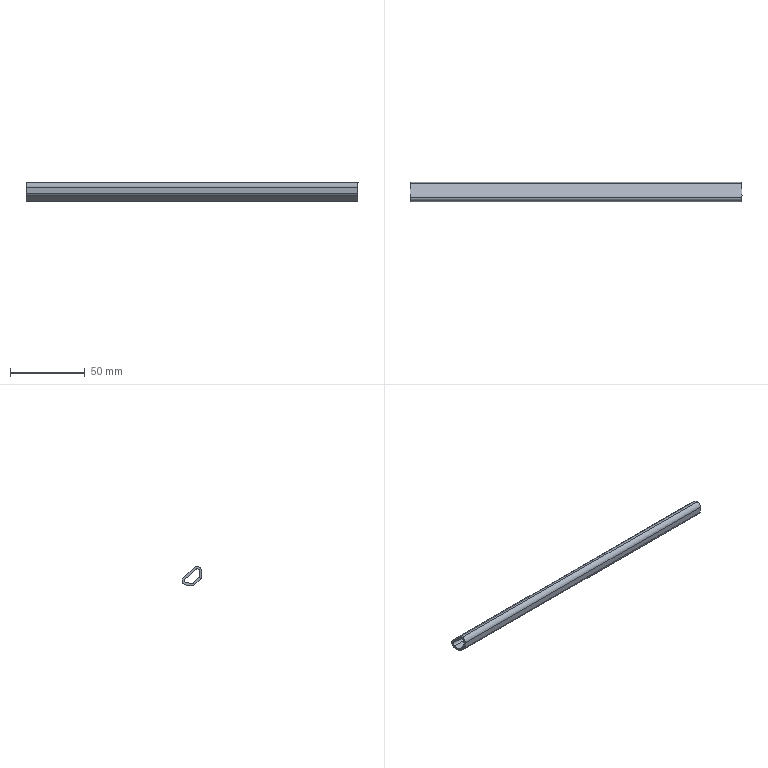Part | SolidWorks | features BaseBody 1 | 1 solid | 20 faces | box 221.8 x 13.077 x 12.577 mm | volume 11773 mm3 | plane 10 | cylinder 10 | commonest cylinder face diameters 3 x3 6 x3 1 x2 4 x2
STEP:
#1=CARTESIAN_POINT('',(110.837,-148.389,-339.63));
#2=VERTEX_POINT('',#1);
#3=CARTESIAN_POINT('',(-110.963,-148.389,-339.63));
#4=VERTEX_POINT('',#3);
#5=CARTESIAN_POINT('',(110.837,-148.389,-339.63));
#6=DIRECTION('',(-1.,0.000000003,0.000000006));
#7=VECTOR('',#6,1000.);
#8=LINE('',#5,#7);
#9=EDGE_CURVE('',#2,#4,#8,.T.);
#10=ORIENTED_EDGE('',*,*,#9,.F.);
#11=CARTESIAN_POINT('',(110.837,-144.347,-339.415));
#12=VERTEX_POINT('',#11);
#13=CARTESIAN_POINT('',(110.837,-144.347,-339.415));
#14=DIRECTION('',(-0.000000003,-0.9986,-0.05296));
#15=VECTOR('',#14,1000.);
#16=LINE('',#13,#15);
#17=EDGE_CURVE('',#12,#2,#16,.T.);
#18=ORIENTED_EDGE('',*,*,#17,.F.);
#19=CARTESIAN_POINT('',(-110.963,-144.347,-339.415));
#20=VERTEX_POINT('',#19);
#21=CARTESIAN_POINT('',(110.837,-144.347,-339.415));
#22=DIRECTION('',(-1.,0.000000003,0.000000006));
#23=VECTOR('',#22,1000.);
#24=LINE('',#21,#23);
#25=EDGE_CURVE('',#12,#20,#24,.T.);
#26=ORIENTED_EDGE('',*,*,#25,.T.);
#27=CARTESIAN_POINT('',(-110.963,-144.347,-339.415));
#28=DIRECTION('',(-0.000000003,-0.9986,-0.05296));
#29=VECTOR('',#28,1000.);
#30=LINE('',#27,#29);
#31=EDGE_CURVE('',#20,#4,#30,.T.);
#32=ORIENTED_EDGE('',*,*,#31,.T.);
#33=EDGE_LOOP('',(#10,#18,#26,#32));
#34=FACE_OUTER_BOUND('',#33,.T.);
#35=CARTESIAN_POINT('',(-110.563,-144.347,-339.415));
#36=DIRECTION('',(0.000000006,-0.05296,0.9986));
#37=DIRECTION('',(-1.,-0.000000113,0.));
#38=AXIS2_PLACEMENT_3D('',#35,#36,#37);
#39=PLANE('',#38);
#40=ADVANCED_FACE('',(#34),#39,.T.);
#41=CARTESIAN_POINT('',(-110.963,-150.5,-330.438));
#42=VERTEX_POINT('',#41);
#43=CARTESIAN_POINT('',(-110.963,-143.423,-336.802));
#44=VERTEX_POINT('',#43);
#45=CARTESIAN_POINT('',(-110.963,-150.5,-330.438));
#46=DIRECTION('',(-0.000000002,0.7436,-0.6687));
#47=VECTOR('',#46,1000.);
#48=LINE('',#45,#47);
#49=EDGE_CURVE('',#42,#44,#48,.T.);
#50=ORIENTED_EDGE('',*,*,#49,.F.);
#51=CARTESIAN_POINT('',(-110.963,-151.583,-330.055));
#52=VERTEX_POINT('',#51);
#53=CARTESIAN_POINT('',(-110.963,-151.503,-331.553));
#54=DIRECTION('',(-1.,0.000000003,0.000000006));
#55=DIRECTION('',(0.000000006,-0.05296,0.9986));
#56=AXIS2_PLACEMENT_3D('',#53,#54,#55);
#57=CIRCLE('',#56,1.5);
#58=EDGE_CURVE('',#52,#42,#57,.T.);
#59=ORIENTED_EDGE('',*,*,#58,.F.);
#60=CARTESIAN_POINT('',(-110.963,-153.001,-331.633));
#61=VERTEX_POINT('',#60);
#62=CARTESIAN_POINT('',(-110.963,-151.503,-331.553));
#63=DIRECTION('',(-1.,0.000000003,0.000000006));
#64=DIRECTION('',(0.000000006,-0.05296,0.9986));
#65=AXIS2_PLACEMENT_3D('',#62,#63,#64);
#66=CIRCLE('',#65,1.5);
#67=EDGE_CURVE('',#61,#52,#66,.T.);
#68=ORIENTED_EDGE('',*,*,#67,.F.);
#69=CARTESIAN_POINT('',(-110.963,-152.787,-335.675));
#70=VERTEX_POINT('',#69);
#71=CARTESIAN_POINT('',(-110.963,-152.787,-335.675));
#72=DIRECTION('',(0.000000006,-0.05296,0.9986));
#73=VECTOR('',#72,1000.);
#74=LINE('',#71,#73);
#75=EDGE_CURVE('',#70,#61,#74,.T.);
#76=ORIENTED_EDGE('',*,*,#75,.F.);
#77=CARTESIAN_POINT('',(-110.963,-152.622,-336.021));
#78=VERTEX_POINT('',#77);
#79=CARTESIAN_POINT('',(-110.963,-152.287,-335.649));
#80=DIRECTION('',(-1.,0.000000003,0.000000006));
#81=DIRECTION('',(-0.000000006,-0.6687,-0.7436));
#82=AXIS2_PLACEMENT_3D('',#79,#80,#81);
#83=CIRCLE('',#82,0.5);
#84=EDGE_CURVE('',#78,#70,#83,.T.);
#85=ORIENTED_EDGE('',*,*,#84,.F.);
#86=CARTESIAN_POINT('',(-110.963,-148.75,-339.502));
#87=VERTEX_POINT('',#86);
#88=CARTESIAN_POINT('',(-110.963,-148.75,-339.502));
#89=DIRECTION('',(0.000000002,-0.7436,0.6687));
#90=VECTOR('',#89,1000.);
#91=LINE('',#88,#90);
#92=EDGE_CURVE('',#87,#78,#91,.T.);
#93=ORIENTED_EDGE('',*,*,#92,.F.);
#94=CARTESIAN_POINT('',(-110.963,-148.416,-339.13));
#95=DIRECTION('',(-1.,0.000000003,0.000000006));
#96=DIRECTION('',(-0.000000006,0.05296,-0.9986));
#97=AXIS2_PLACEMENT_3D('',#94,#95,#96);
#98=CIRCLE('',#97,0.5);
#99=EDGE_CURVE('',#4,#87,#98,.T.);
#100=ORIENTED_EDGE('',*,*,#99,.F.);
#101=ORIENTED_EDGE('',*,*,#31,.F.);
#102=CARTESIAN_POINT('',(-110.963,-144.426,-337.917));
#103=DIRECTION('',(-1.,0.000000003,0.000000006));
#104=DIRECTION('',(0.000000006,0.6687,0.7436));
#105=AXIS2_PLACEMENT_3D('',#102,#103,#104);
#106=CIRCLE('',#105,1.5);
#107=EDGE_CURVE('',#44,#20,#106,.T.);
#108=ORIENTED_EDGE('',*,*,#107,.F.);
#109=EDGE_LOOP('',(#50,#59,#68,#76,#85,#93,#100,#101,#108));
#110=FACE_BOUND('',#109,.T.);
#111=CARTESIAN_POINT('',(-110.963,-153.625,-337.136));
#112=VERTEX_POINT('',#111);
#113=CARTESIAN_POINT('',(-110.963,-149.753,-340.618));
#114=VERTEX_POINT('',#113);
#115=CARTESIAN_POINT('',(-110.963,-153.625,-337.136));
#116=DIRECTION('',(-0.000000002,0.7436,-0.6687));
#117=VECTOR('',#116,1000.);
#118=LINE('',#115,#117);
#119=EDGE_CURVE('',#112,#114,#118,.T.);
#120=ORIENTED_EDGE('',*,*,#119,.F.);
#121=CARTESIAN_POINT('',(-110.963,-154.285,-335.755));
#122=VERTEX_POINT('',#121);
#123=CARTESIAN_POINT('',(-110.963,-152.287,-335.649));
#124=DIRECTION('',(1.,-0.000000003,-0.000000006));
#125=DIRECTION('',(-0.000000003,-0.9986,-0.05296));
#126=AXIS2_PLACEMENT_3D('',#123,#124,#125);
#127=CIRCLE('',#126,2.);
#128=EDGE_CURVE('',#122,#112,#127,.T.);
#129=ORIENTED_EDGE('',*,*,#128,.F.);
#130=CARTESIAN_POINT('',(-110.963,-154.499,-331.712));
#131=VERTEX_POINT('',#130);
#132=CARTESIAN_POINT('',(-110.963,-154.499,-331.712));
#133=DIRECTION('',(-0.000000006,0.05296,-0.9986));
#134=VECTOR('',#133,1000.);
#135=LINE('',#132,#134);
#136=EDGE_CURVE('',#131,#122,#135,.T.);
#137=ORIENTED_EDGE('',*,*,#136,.F.);
#138=CARTESIAN_POINT('',(-110.963,-151.662,-328.557));
#139=VERTEX_POINT('',#138);
#140=CARTESIAN_POINT('',(-110.963,-151.503,-331.553));
#141=DIRECTION('',(1.,-0.000000003,-0.000000006));
#142=DIRECTION('',(0.000000006,-0.05296,0.9986));
#143=AXIS2_PLACEMENT_3D('',#140,#141,#142);
#144=CIRCLE('',#143,3.);
#145=EDGE_CURVE('',#139,#131,#144,.T.);
#146=ORIENTED_EDGE('',*,*,#145,.F.);
#147=CARTESIAN_POINT('',(-110.963,-149.497,-329.323));
#148=VERTEX_POINT('',#147);
#149=CARTESIAN_POINT('',(-110.963,-151.503,-331.553));
#150=DIRECTION('',(1.,-0.000000003,-0.000000006));
#151=DIRECTION('',(0.000000006,0.6687,0.7436));
#152=AXIS2_PLACEMENT_3D('',#149,#150,#151);
#153=CIRCLE('',#152,3.);
#154=EDGE_CURVE('',#148,#139,#153,.T.);
#155=ORIENTED_EDGE('',*,*,#154,.F.);
#156=CARTESIAN_POINT('',(-110.963,-142.42,-335.687));
#157=VERTEX_POINT('',#156);
#158=CARTESIAN_POINT('',(-110.963,-142.42,-335.687));
#159=DIRECTION('',(0.000000002,-0.7436,0.6687));
#160=VECTOR('',#159,1000.);
#161=LINE('',#158,#160);
#162=EDGE_CURVE('',#157,#148,#161,.T.);
#163=ORIENTED_EDGE('',*,*,#162,.F.);
#164=CARTESIAN_POINT('',(-110.963,-144.267,-340.913));
#165=VERTEX_POINT('',#164);
#166=CARTESIAN_POINT('',(-110.963,-144.426,-337.917));
#167=DIRECTION('',(1.,-0.000000003,-0.000000006));
#168=DIRECTION('',(-0.000000006,0.05296,-0.9986));
#169=AXIS2_PLACEMENT_3D('',#166,#167,#168);
#170=CIRCLE('',#169,3.);
#171=EDGE_CURVE('',#165,#157,#170,.T.);
#172=ORIENTED_EDGE('',*,*,#171,.F.);
#173=CARTESIAN_POINT('',(-110.963,-148.31,-341.128));
#174=VERTEX_POINT('',#173);
#175=CARTESIAN_POINT('',(-110.963,-148.31,-341.128));
#176=DIRECTION('',(0.000000003,0.9986,0.05296));
#177=VECTOR('',#176,1000.);
#178=LINE('',#175,#177);
#179=EDGE_CURVE('',#174,#165,#178,.T.);
#180=ORIENTED_EDGE('',*,*,#179,.F.);
#181=CARTESIAN_POINT('',(-110.963,-148.416,-339.13));
#182=DIRECTION('',(1.,-0.000000003,-0.000000006));
#183=DIRECTION('',(-0.000000006,-0.6687,-0.7436));
#184=AXIS2_PLACEMENT_3D('',#181,#182,#183);
#185=CIRCLE('',#184,2.);
#186=EDGE_CURVE('',#114,#174,#185,.T.);
#187=ORIENTED_EDGE('',*,*,#186,.F.);
#188=EDGE_LOOP('',(#120,#129,#137,#146,#155,#163,#172,#180,#187));
#189=FACE_OUTER_BOUND('',#188,.T.);
#190=CARTESIAN_POINT('',(-110.963,-148.416,-339.13));
#191=DIRECTION('',(1.,-0.000000003,-0.000000006));
#192=DIRECTION('',(0.,-0.9065,0.4222));
#193=AXIS2_PLACEMENT_3D('',#190,#191,#192);
#194=PLANE('',#193);
#195=ADVANCED_FACE('',(#110,#189),#194,.F.);
#196=CARTESIAN_POINT('',(110.837,-149.753,-340.618));
#197=VERTEX_POINT('',#196);
#198=CARTESIAN_POINT('',(110.837,-149.753,-340.618));
#199=DIRECTION('',(-1.,0.000000003,0.000000006));
#200=VECTOR('',#199,1000.);
#201=LINE('',#198,#200);
#202=EDGE_CURVE('',#197,#114,#201,.T.);
#203=ORIENTED_EDGE('',*,*,#202,.T.);
#204=ORIENTED_EDGE('',*,*,#186,.T.);
#205=CARTESIAN_POINT('',(110.837,-148.31,-341.128));
#206=VERTEX_POINT('',#205);
#207=CARTESIAN_POINT('',(110.837,-148.31,-341.128));
#208=DIRECTION('',(-1.,0.000000003,0.000000006));
#209=VECTOR('',#208,1000.);
#210=LINE('',#207,#209);
#211=EDGE_CURVE('',#206,#174,#210,.T.);
#212=ORIENTED_EDGE('',*,*,#211,.F.);
#213=CARTESIAN_POINT('',(110.837,-148.416,-339.13));
#214=DIRECTION('',(-1.,0.000000003,0.000000006));
#215=DIRECTION('',(-0.000000006,0.05296,-0.9986));
#216=AXIS2_PLACEMENT_3D('',#213,#214,#215);
#217=CIRCLE('',#216,2.);
#218=EDGE_CURVE('',#206,#197,#217,.T.);
#219=ORIENTED_EDGE('',*,*,#218,.T.);
#220=EDGE_LOOP('',(#203,#204,#212,#219));
#221=FACE_OUTER_BOUND('',#220,.T.);
#222=CARTESIAN_POINT('',(-110.563,-148.416,-339.13));
#223=DIRECTION('',(1.,-0.000000003,-0.000000006));
#224=DIRECTION('',(0.000000006,-0.05296,0.9986));
#225=AXIS2_PLACEMENT_3D('',#222,#223,#224);
#226=CYLINDRICAL_SURFACE('',#225,2.);
#227=ADVANCED_FACE('',(#221),#226,.T.);
#228=ORIENTED_EDGE('',*,*,#17,.T.);
#229=CARTESIAN_POINT('',(110.837,-148.75,-339.502));
#230=VERTEX_POINT('',#229);
#231=CARTESIAN_POINT('',(110.837,-148.416,-339.13));
#232=DIRECTION('',(1.,-0.000000003,-0.000000006));
#233=DIRECTION('',(-0.000000006,-0.6687,-0.7436));
#234=AXIS2_PLACEMENT_3D('',#231,#232,#233);
#235=CIRCLE('',#234,0.5);
#236=EDGE_CURVE('',#230,#2,#235,.T.);
#237=ORIENTED_EDGE('',*,*,#236,.F.);
#238=CARTESIAN_POINT('',(110.837,-152.622,-336.021));
#239=VERTEX_POINT('',#238);
#240=CARTESIAN_POINT('',(110.837,-152.622,-336.021));
#241=DIRECTION('',(-0.000000002,0.7436,-0.6687));
#242=VECTOR('',#241,1000.);
#243=LINE('',#240,#242);
#244=EDGE_CURVE('',#239,#230,#243,.T.);
#245=ORIENTED_EDGE('',*,*,#244,.F.);
#246=CARTESIAN_POINT('',(110.837,-152.787,-335.675));
#247=VERTEX_POINT('',#246);
#248=CARTESIAN_POINT('',(110.837,-152.287,-335.649));
#249=DIRECTION('',(1.,-0.000000003,-0.000000006));
#250=DIRECTION('',(-0.000000003,-0.9986,-0.05296));
#251=AXIS2_PLACEMENT_3D('',#248,#249,#250);
#252=CIRCLE('',#251,0.5);
#253=EDGE_CURVE('',#247,#239,#252,.T.);
#254=ORIENTED_EDGE('',*,*,#253,.F.);
#255=CARTESIAN_POINT('',(110.837,-153.001,-331.633));
#256=VERTEX_POINT('',#255);
#257=CARTESIAN_POINT('',(110.837,-152.787,-335.675));
#258=DIRECTION('',(0.000000006,-0.05296,0.9986));
#259=VECTOR('',#258,1000.);
#260=LINE('',#257,#259);
#261=EDGE_CURVE('',#247,#256,#260,.T.);
#262=ORIENTED_EDGE('',*,*,#261,.T.);
#263=CARTESIAN_POINT('',(110.837,-151.583,-330.055));
#264=VERTEX_POINT('',#263);
#265=CARTESIAN_POINT('',(110.837,-151.503,-331.553));
#266=DIRECTION('',(1.,-0.000000003,-0.000000006));
#267=DIRECTION('',(0.000000006,-0.05296,0.9986));
#268=AXIS2_PLACEMENT_3D('',#265,#266,#267);
#269=CIRCLE('',#268,1.5);
#270=EDGE_CURVE('',#264,#256,#269,.T.);
#271=ORIENTED_EDGE('',*,*,#270,.F.);
#272=CARTESIAN_POINT('',(110.837,-150.5,-330.438));
#273=VERTEX_POINT('',#272);
#274=CARTESIAN_POINT('',(110.837,-151.503,-331.553));
#275=DIRECTION('',(1.,-0.000000003,-0.000000006));
#276=DIRECTION('',(0.000000006,-0.05296,0.9986));
#277=AXIS2_PLACEMENT_3D('',#274,#275,#276);
#278=CIRCLE('',#277,1.5);
#279=EDGE_CURVE('',#273,#264,#278,.T.);
#280=ORIENTED_EDGE('',*,*,#279,.F.);
#281=CARTESIAN_POINT('',(110.837,-143.423,-336.802));
#282=VERTEX_POINT('',#281);
#283=CARTESIAN_POINT('',(110.837,-143.423,-336.802));
#284=DIRECTION('',(0.000000002,-0.7436,0.6687));
#285=VECTOR('',#284,1000.);
#286=LINE('',#283,#285);
#287=EDGE_CURVE('',#282,#273,#286,.T.);
#288=ORIENTED_EDGE('',*,*,#287,.F.);
#289=CARTESIAN_POINT('',(110.837,-144.426,-337.917));
#290=DIRECTION('',(1.,-0.000000003,-0.000000006));
#291=DIRECTION('',(-0.000000006,0.05296,-0.9986));
#292=AXIS2_PLACEMENT_3D('',#289,#290,#291);
#293=CIRCLE('',#292,1.5);
#294=EDGE_CURVE('',#12,#282,#293,.T.);
#295=ORIENTED_EDGE('',*,*,#294,.F.);
#296=EDGE_LOOP('',(#228,#237,#245,#254,#262,#271,#280,#288,#295));
#297=FACE_BOUND('',#296,.T.);
#298=CARTESIAN_POINT('',(110.837,-144.267,-340.913));
#299=VERTEX_POINT('',#298);
#300=CARTESIAN_POINT('',(110.837,-148.31,-341.128));
#301=DIRECTION('',(0.000000003,0.9986,0.05296));
#302=VECTOR('',#301,1000.);
#303=LINE('',#300,#302);
#304=EDGE_CURVE('',#206,#299,#303,.T.);
#305=ORIENTED_EDGE('',*,*,#304,.T.);
#306=CARTESIAN_POINT('',(110.837,-142.42,-335.687));
#307=VERTEX_POINT('',#306);
#308=CARTESIAN_POINT('',(110.837,-144.426,-337.917));
#309=DIRECTION('',(-1.,0.000000003,0.000000006));
#310=DIRECTION('',(0.000000006,0.6687,0.7436));
#311=AXIS2_PLACEMENT_3D('',#308,#309,#310);
#312=CIRCLE('',#311,3.);
#313=EDGE_CURVE('',#307,#299,#312,.T.);
#314=ORIENTED_EDGE('',*,*,#313,.F.);
#315=CARTESIAN_POINT('',(110.837,-149.497,-329.323));
#316=VERTEX_POINT('',#315);
#317=CARTESIAN_POINT('',(110.837,-149.497,-329.323));
#318=DIRECTION('',(-0.000000002,0.7436,-0.6687));
#319=VECTOR('',#318,1000.);
#320=LINE('',#317,#319);
#321=EDGE_CURVE('',#316,#307,#320,.T.);
#322=ORIENTED_EDGE('',*,*,#321,.F.);
#323=CARTESIAN_POINT('',(110.837,-151.662,-328.557));
#324=VERTEX_POINT('',#323);
#325=CARTESIAN_POINT('',(110.837,-151.503,-331.553));
#326=DIRECTION('',(-1.,0.000000003,0.000000006));
#327=DIRECTION('',(0.000000006,-0.05296,0.9986));
#328=AXIS2_PLACEMENT_3D('',#325,#326,#327);
#329=CIRCLE('',#328,3.);
#330=EDGE_CURVE('',#324,#316,#329,.T.);
#331=ORIENTED_EDGE('',*,*,#330,.F.);
#332=CARTESIAN_POINT('',(110.837,-154.499,-331.712));
#333=VERTEX_POINT('',#332);
#334=CARTESIAN_POINT('',(110.837,-151.503,-331.553));
#335=DIRECTION('',(-1.,0.000000003,0.000000006));
#336=DIRECTION('',(-0.000000003,-0.9986,-0.05296));
#337=AXIS2_PLACEMENT_3D('',#334,#335,#336);
#338=CIRCLE('',#337,3.);
#339=EDGE_CURVE('',#333,#324,#338,.T.);
#340=ORIENTED_EDGE('',*,*,#339,.F.);
#341=CARTESIAN_POINT('',(110.837,-154.285,-335.755));
#342=VERTEX_POINT('',#341);
#343=CARTESIAN_POINT('',(110.837,-154.499,-331.712));
#344=DIRECTION('',(-0.000000006,0.05296,-0.9986));
#345=VECTOR('',#344,1000.);
#346=LINE('',#343,#345);
#347=EDGE_CURVE('',#333,#342,#346,.T.);
#348=ORIENTED_EDGE('',*,*,#347,.T.);
#349=CARTESIAN_POINT('',(110.837,-153.625,-337.136));
#350=VERTEX_POINT('',#349);
#351=CARTESIAN_POINT('',(110.837,-152.287,-335.649));
#352=DIRECTION('',(-1.,0.000000003,0.000000006));
#353=DIRECTION('',(-0.000000006,-0.6687,-0.7436));
#354=AXIS2_PLACEMENT_3D('',#351,#352,#353);
#355=CIRCLE('',#354,2.);
#356=EDGE_CURVE('',#350,#342,#355,.T.);
#357=ORIENTED_EDGE('',*,*,#356,.F.);
#358=CARTESIAN_POINT('',(110.837,-149.753,-340.618));
#359=DIRECTION('',(0.000000002,-0.7436,0.6687));
#360=VECTOR('',#359,1000.);
#361=LINE('',#358,#360);
#362=EDGE_CURVE('',#197,#350,#361,.T.);
#363=ORIENTED_EDGE('',*,*,#362,.F.);
#364=ORIENTED_EDGE('',*,*,#218,.F.);
#365=EDGE_LOOP('',(#305,#314,#322,#331,#340,#348,#357,#363,#364));
#366=FACE_OUTER_BOUND('',#365,.T.);
#367=CARTESIAN_POINT('',(110.837,-148.416,-339.13));
#368=DIRECTION('',(1.,-0.000000003,-0.000000006));
#369=DIRECTION('',(0.,-0.9065,0.4222));
#370=AXIS2_PLACEMENT_3D('',#367,#368,#369);
#371=PLANE('',#370);
#372=ADVANCED_FACE('',(#297,#366),#371,.T.);
#373=CARTESIAN_POINT('',(110.837,-153.625,-337.136));
#374=DIRECTION('',(-1.,0.000000003,0.000000006));
#375=VECTOR('',#374,1000.);
#376=LINE('',#373,#375);
#377=EDGE_CURVE('',#350,#112,#376,.T.);
#378=ORIENTED_EDGE('',*,*,#377,.T.);
#379=ORIENTED_EDGE('',*,*,#119,.T.);
#380=ORIENTED_EDGE('',*,*,#202,.F.);
#381=ORIENTED_EDGE('',*,*,#362,.T.);
#382=EDGE_LOOP('',(#378,#379,#380,#381));
#383=FACE_OUTER_BOUND('',#382,.T.);
#384=CARTESIAN_POINT('',(-110.563,-149.753,-340.618));
#385=DIRECTION('',(0.000000006,0.6687,0.7436));
#386=DIRECTION('',(1.,-0.00000001,0.));
#387=AXIS2_PLACEMENT_3D('',#384,#385,#386);
#388=PLANE('',#387);
#389=ADVANCED_FACE('',(#383),#388,.F.);
#390=CARTESIAN_POINT('',(110.837,-154.285,-335.755));
#391=DIRECTION('',(-1.,0.000000003,0.000000006));
#392=VECTOR('',#391,1000.);
#393=LINE('',#390,#392);
#394=EDGE_CURVE('',#342,#122,#393,.T.);
#395=ORIENTED_EDGE('',*,*,#394,.T.);
#396=ORIENTED_EDGE('',*,*,#128,.T.);
#397=ORIENTED_EDGE('',*,*,#377,.F.);
#398=ORIENTED_EDGE('',*,*,#356,.T.);
#399=EDGE_LOOP('',(#395,#396,#397,#398));
#400=FACE_OUTER_BOUND('',#399,.T.);
#401=CARTESIAN_POINT('',(-110.563,-152.287,-335.649));
#402=DIRECTION('',(1.,-0.000000003,-0.000000006));
#403=DIRECTION('',(0.000000006,-0.05296,0.9986));
#404=AXIS2_PLACEMENT_3D('',#401,#402,#403);
#405=CYLINDRICAL_SURFACE('',#404,2.);
#406=ADVANCED_FACE('',(#400),#405,.T.);
#407=CARTESIAN_POINT('',(110.837,-154.499,-331.712));
#408=DIRECTION('',(-1.,0.000000003,0.000000006));
#409=VECTOR('',#408,1000.);
#410=LINE('',#407,#409);
#411=EDGE_CURVE('',#333,#131,#410,.T.);
#412=ORIENTED_EDGE('',*,*,#411,.T.);
#413=ORIENTED_EDGE('',*,*,#136,.T.);
#414=ORIENTED_EDGE('',*,*,#394,.F.);
#415=ORIENTED_EDGE('',*,*,#347,.F.);
#416=EDGE_LOOP('',(#412,#413,#414,#415));
#417=FACE_OUTER_BOUND('',#416,.T.);
#418=CARTESIAN_POINT('',(-110.563,-154.285,-335.755));
#419=DIRECTION('',(0.000000003,0.9986,0.05296));
#420=DIRECTION('',(1.,0.,-0.00000006));
#421=AXIS2_PLACEMENT_3D('',#418,#419,#420);
#422=PLANE('',#421);
#423=ADVANCED_FACE('',(#417),#422,.F.);
#424=ORIENTED_EDGE('',*,*,#145,.T.);
#425=ORIENTED_EDGE('',*,*,#411,.F.);
#426=ORIENTED_EDGE('',*,*,#339,.T.);
#427=CARTESIAN_POINT('',(110.837,-151.662,-328.557));
#428=DIRECTION('',(-1.,0.000000003,0.000000006));
#429=VECTOR('',#428,1000.);
#430=LINE('',#427,#429);
#431=EDGE_CURVE('',#324,#139,#430,.T.);
#432=ORIENTED_EDGE('',*,*,#431,.T.);
#433=EDGE_LOOP('',(#424,#425,#426,#432));
#434=FACE_OUTER_BOUND('',#433,.T.);
#435=CARTESIAN_POINT('',(-110.563,-151.503,-331.553));
#436=DIRECTION('',(1.,-0.000000003,-0.000000006));
#437=DIRECTION('',(0.000000006,-0.05296,0.9986));
#438=AXIS2_PLACEMENT_3D('',#435,#436,#437);
#439=CYLINDRICAL_SURFACE('',#438,3.);
#440=ADVANCED_FACE('',(#434),#439,.T.);
#441=ORIENTED_EDGE('',*,*,#431,.F.);
#442=ORIENTED_EDGE('',*,*,#330,.T.);
#443=CARTESIAN_POINT('',(110.837,-149.497,-329.323));
#444=DIRECTION('',(-1.,0.000000003,0.000000006));
#445=VECTOR('',#444,1000.);
#446=LINE('',#443,#445);
#447=EDGE_CURVE('',#316,#148,#446,.T.);
#448=ORIENTED_EDGE('',*,*,#447,.T.);
#449=ORIENTED_EDGE('',*,*,#154,.T.);
#450=EDGE_LOOP('',(#441,#442,#448,#449));
#451=FACE_OUTER_BOUND('',#450,.T.);
#452=CARTESIAN_POINT('',(-110.563,-151.503,-331.553));
#453=DIRECTION('',(1.,-0.000000003,-0.000000006));
#454=DIRECTION('',(0.000000006,-0.05296,0.9986));
#455=AXIS2_PLACEMENT_3D('',#452,#453,#454);
#456=CYLINDRICAL_SURFACE('',#455,3.);
#457=ADVANCED_FACE('',(#451),#456,.T.);
#458=CARTESIAN_POINT('',(110.837,-142.42,-335.687));
#459=DIRECTION('',(-1.,0.000000003,0.000000006));
#460=VECTOR('',#459,1000.);
#461=LINE('',#458,#460);
#462=EDGE_CURVE('',#307,#157,#461,.T.);
#463=ORIENTED_EDGE('',*,*,#462,.T.);
#464=ORIENTED_EDGE('',*,*,#162,.T.);
#465=ORIENTED_EDGE('',*,*,#447,.F.);
#466=ORIENTED_EDGE('',*,*,#321,.T.);
#467=EDGE_LOOP('',(#463,#464,#465,#466));
#468=FACE_OUTER_BOUND('',#467,.T.);
#469=CARTESIAN_POINT('',(-110.563,-142.42,-335.687));
#470=DIRECTION('',(0.000000006,0.6687,0.7436));
#471=DIRECTION('',(1.,-0.00000001,0.));
#472=AXIS2_PLACEMENT_3D('',#469,#470,#471);
#473=PLANE('',#472);
#474=ADVANCED_FACE('',(#468),#473,.T.);
#475=CARTESIAN_POINT('',(110.837,-144.267,-340.913));
#476=DIRECTION('',(-1.,0.000000003,0.000000006));
#477=VECTOR('',#476,1000.);
#478=LINE('',#475,#477);
#479=EDGE_CURVE('',#299,#165,#478,.T.);
#480=ORIENTED_EDGE('',*,*,#479,.T.);
#481=ORIENTED_EDGE('',*,*,#171,.T.);
#482=ORIENTED_EDGE('',*,*,#462,.F.);
#483=ORIENTED_EDGE('',*,*,#313,.T.);
#484=EDGE_LOOP('',(#480,#481,#482,#483));
#485=FACE_OUTER_BOUND('',#484,.T.);
#486=CARTESIAN_POINT('',(-110.563,-144.426,-337.917));
#487=DIRECTION('',(1.,-0.000000003,-0.000000006));
#488=DIRECTION('',(0.000000006,-0.05296,0.9986));
#489=AXIS2_PLACEMENT_3D('',#486,#487,#488);
#490=CYLINDRICAL_SURFACE('',#489,3.);
#491=ADVANCED_FACE('',(#485),#490,.T.);
#492=ORIENTED_EDGE('',*,*,#211,.T.);
#493=ORIENTED_EDGE('',*,*,#179,.T.);
#494=ORIENTED_EDGE('',*,*,#479,.F.);
#495=ORIENTED_EDGE('',*,*,#304,.F.);
#496=EDGE_LOOP('',(#492,#493,#494,#495));
#497=FACE_OUTER_BOUND('',#496,.T.);
#498=CARTESIAN_POINT('',(-110.563,-144.267,-340.913));
#499=DIRECTION('',(0.000000006,-0.05296,0.9986));
#500=DIRECTION('',(-1.,-0.000000113,0.));
#501=AXIS2_PLACEMENT_3D('',#498,#499,#500);
#502=PLANE('',#501);
#503=ADVANCED_FACE('',(#497),#502,.F.);
#504=ORIENTED_EDGE('',*,*,#25,.F.);
#505=ORIENTED_EDGE('',*,*,#294,.T.);
#506=CARTESIAN_POINT('',(110.837,-143.423,-336.802));
#507=DIRECTION('',(-1.,0.000000003,0.000000006));
#508=VECTOR('',#507,1000.);
#509=LINE('',#506,#508);
#510=EDGE_CURVE('',#282,#44,#509,.T.);
#511=ORIENTED_EDGE('',*,*,#510,.T.);
#512=ORIENTED_EDGE('',*,*,#107,.T.);
#513=EDGE_LOOP('',(#504,#505,#511,#512));
#514=FACE_OUTER_BOUND('',#513,.T.);
#515=CARTESIAN_POINT('',(-110.563,-144.426,-337.917));
#516=DIRECTION('',(1.,-0.000000003,-0.000000006));
#517=DIRECTION('',(0.000000006,-0.05296,0.9986));
#518=AXIS2_PLACEMENT_3D('',#515,#516,#517);
#519=CYLINDRICAL_SURFACE('',#518,1.5);
#520=ADVANCED_FACE('',(#514),#519,.F.);
#521=ORIENTED_EDGE('',*,*,#510,.F.);
#522=ORIENTED_EDGE('',*,*,#287,.T.);
#523=CARTESIAN_POINT('',(110.837,-150.5,-330.438));
#524=DIRECTION('',(-1.,0.000000003,0.000000006));
#525=VECTOR('',#524,1000.);
#526=LINE('',#523,#525);
#527=EDGE_CURVE('',#273,#42,#526,.T.);
#528=ORIENTED_EDGE('',*,*,#527,.T.);
#529=ORIENTED_EDGE('',*,*,#49,.T.);
#530=EDGE_LOOP('',(#521,#522,#528,#529));
#531=FACE_OUTER_BOUND('',#530,.T.);
#532=CARTESIAN_POINT('',(-110.563,-143.423,-336.802));
#533=DIRECTION('',(0.000000006,0.6687,0.7436));
#534=DIRECTION('',(1.,-0.00000001,0.));
#535=AXIS2_PLACEMENT_3D('',#532,#533,#534);
#536=PLANE('',#535);
#537=ADVANCED_FACE('',(#531),#536,.F.);
#538=CARTESIAN_POINT('',(-110.563,-151.583,-330.055));
#539=DIRECTION('',(1.,-0.000000003,-0.000000006));
#540=VECTOR('',#539,1000.);
#541=LINE('',#538,#540);
#542=EDGE_CURVE('',#52,#264,#541,.T.);
#543=ORIENTED_EDGE('',*,*,#542,.F.);
#544=ORIENTED_EDGE('',*,*,#58,.T.);
#545=ORIENTED_EDGE('',*,*,#527,.F.);
#546=ORIENTED_EDGE('',*,*,#279,.T.);
#547=EDGE_LOOP('',(#543,#544,#545,#546));
#548=FACE_OUTER_BOUND('',#547,.T.);
#549=CARTESIAN_POINT('',(-110.563,-151.503,-331.553));
#550=DIRECTION('',(1.,-0.000000003,-0.000000006));
#551=DIRECTION('',(0.000000006,-0.05296,0.9986));
#552=AXIS2_PLACEMENT_3D('',#549,#550,#551);
#553=CYLINDRICAL_SURFACE('',#552,1.5);
#554=ADVANCED_FACE('',(#548),#553,.F.);
#555=CARTESIAN_POINT('',(110.837,-153.001,-331.633));
#556=DIRECTION('',(-1.,0.000000003,0.000000006));
#557=VECTOR('',#556,1000.);
#558=LINE('',#555,#557);
#559=EDGE_CURVE('',#256,#61,#558,.T.);
#560=ORIENTED_EDGE('',*,*,#559,.F.);
#561=ORIENTED_EDGE('',*,*,#261,.F.);
#562=CARTESIAN_POINT('',(110.837,-152.787,-335.675));
#563=DIRECTION('',(-1.,0.000000003,0.000000006));
#564=VECTOR('',#563,1000.);
#565=LINE('',#562,#564);
#566=EDGE_CURVE('',#247,#70,#565,.T.);
#567=ORIENTED_EDGE('',*,*,#566,.T.);
#568=ORIENTED_EDGE('',*,*,#75,.T.);
#569=EDGE_LOOP('',(#560,#561,#567,#568));
#570=FACE_OUTER_BOUND('',#569,.T.);
#571=CARTESIAN_POINT('',(-110.563,-152.787,-335.675));
#572=DIRECTION('',(0.000000003,0.9986,0.05296));
#573=DIRECTION('',(1.,0.,-0.00000006));
#574=AXIS2_PLACEMENT_3D('',#571,#572,#573);
#575=PLANE('',#574);
#576=ADVANCED_FACE('',(#570),#575,.T.);
#577=ORIENTED_EDGE('',*,*,#566,.F.);
#578=ORIENTED_EDGE('',*,*,#253,.T.);
#579=CARTESIAN_POINT('',(110.837,-152.622,-336.021));
#580=DIRECTION('',(-1.,0.000000003,0.000000006));
#581=VECTOR('',#580,1000.);
#582=LINE('',#579,#581);
#583=EDGE_CURVE('',#239,#78,#582,.T.);
#584=ORIENTED_EDGE('',*,*,#583,.T.);
#585=ORIENTED_EDGE('',*,*,#84,.T.);
#586=EDGE_LOOP('',(#577,#578,#584,#585));
#587=FACE_OUTER_BOUND('',#586,.T.);
#588=CARTESIAN_POINT('',(-110.563,-152.287,-335.649));
#589=DIRECTION('',(1.,-0.000000003,-0.000000006));
#590=DIRECTION('',(0.000000006,-0.05296,0.9986));
#591=AXIS2_PLACEMENT_3D('',#588,#589,#590);
#592=CYLINDRICAL_SURFACE('',#591,0.5);
#593=ADVANCED_FACE('',(#587),#592,.F.);
#594=ORIENTED_EDGE('',*,*,#583,.F.);
#595=ORIENTED_EDGE('',*,*,#244,.T.);
#596=CARTESIAN_POINT('',(110.837,-148.75,-339.502));
#597=DIRECTION('',(-1.,0.000000003,0.000000006));
#598=VECTOR('',#597,1000.);
#599=LINE('',#596,#598);
#600=EDGE_CURVE('',#230,#87,#599,.T.);
#601=ORIENTED_EDGE('',*,*,#600,.T.);
#602=ORIENTED_EDGE('',*,*,#92,.T.);
#603=EDGE_LOOP('',(#594,#595,#601,#602));
#604=FACE_OUTER_BOUND('',#603,.T.);
#605=CARTESIAN_POINT('',(-110.563,-148.75,-339.502));
#606=DIRECTION('',(0.000000006,0.6687,0.7436));
#607=DIRECTION('',(1.,-0.00000001,0.));
#608=AXIS2_PLACEMENT_3D('',#605,#606,#607);
#609=PLANE('',#608);
#610=ADVANCED_FACE('',(#604),#609,.T.);
#611=ORIENTED_EDGE('',*,*,#600,.F.);
#612=ORIENTED_EDGE('',*,*,#236,.T.);
#613=ORIENTED_EDGE('',*,*,#9,.T.);
#614=ORIENTED_EDGE('',*,*,#99,.T.);
#615=EDGE_LOOP('',(#611,#612,#613,#614));
#616=FACE_OUTER_BOUND('',#615,.T.);
#617=CARTESIAN_POINT('',(-110.563,-148.416,-339.13));
#618=DIRECTION('',(1.,-0.000000003,-0.000000006));
#619=DIRECTION('',(0.000000006,-0.05296,0.9986));
#620=AXIS2_PLACEMENT_3D('',#617,#618,#619);
#621=CYLINDRICAL_SURFACE('',#620,0.5);
#622=ADVANCED_FACE('',(#616),#621,.F.);
#623=ORIENTED_EDGE('',*,*,#67,.T.);
#624=ORIENTED_EDGE('',*,*,#542,.T.);
#625=ORIENTED_EDGE('',*,*,#270,.T.);
#626=ORIENTED_EDGE('',*,*,#559,.T.);
#627=EDGE_LOOP('',(#623,#624,#625,#626));
#628=FACE_OUTER_BOUND('',#627,.T.);
#629=CARTESIAN_POINT('',(-110.563,-151.503,-331.553));
#630=DIRECTION('',(1.,-0.000000003,-0.000000006));
#631=DIRECTION('',(0.000000006,-0.05296,0.9986));
#632=AXIS2_PLACEMENT_3D('',#629,#630,#631);
#633=CYLINDRICAL_SURFACE('',#632,1.5);
#634=ADVANCED_FACE('',(#628),#633,.F.);
#635=CLOSED_SHELL('',(#40,#195,#227,#372,#389,#406,#423,#440,#457,#474,#491,#503,#520,#537,#554,#576,#593,#610,#622,#634));
#636=MANIFOLD_SOLID_BREP('',#635);
#637=CARTESIAN_POINT('',(0.,0.,0.));
#638=DIRECTION('',(0.,0.,1.));
#639=DIRECTION('',(1.,0.,0.));
#640=AXIS2_PLACEMENT_3D('',#637,#638,#639);
#641=(LENGTH_UNIT()NAMED_UNIT(*)SI_UNIT(.MILLI.,.METRE.));
#642=UNCERTAINTY_MEASURE_WITH_UNIT(LENGTH_MEASURE(0.00001),#641,'','');
#643=(NAMED_UNIT(*)PLANE_ANGLE_UNIT()SI_UNIT($,.RADIAN.));
#644=(NAMED_UNIT(*)SI_UNIT($,.STERADIAN.)SOLID_ANGLE_UNIT());
#645=(GEOMETRIC_REPRESENTATION_CONTEXT(3)GLOBAL_UNCERTAINTY_ASSIGNED_CONTEXT((#642))GLOBAL_UNIT_ASSIGNED_CONTEXT((#641,#643,#644))REPRESENTATION_CONTEXT('',''));
#646=ADVANCED_BREP_SHAPE_REPRESENTATION('',(#636,#640),#645);